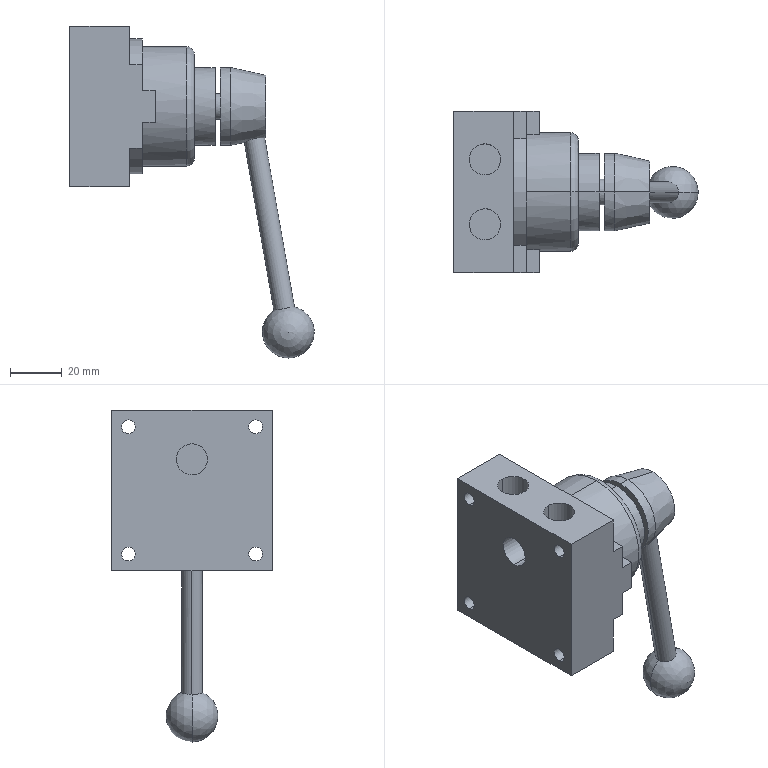Part | STEP file | Positioning_id2222_x_t | 1 solid | 61 faces | box 94.176 x 62 x 127.891 mm | volume 147960 mm3 | cylinder 28 | plane 27 | sphere 2 | cone 2 | torus 2 | commonest cylinder face diameters 5.3 x8 12 x8 30 x4 8 x2 10 x2 46 x2